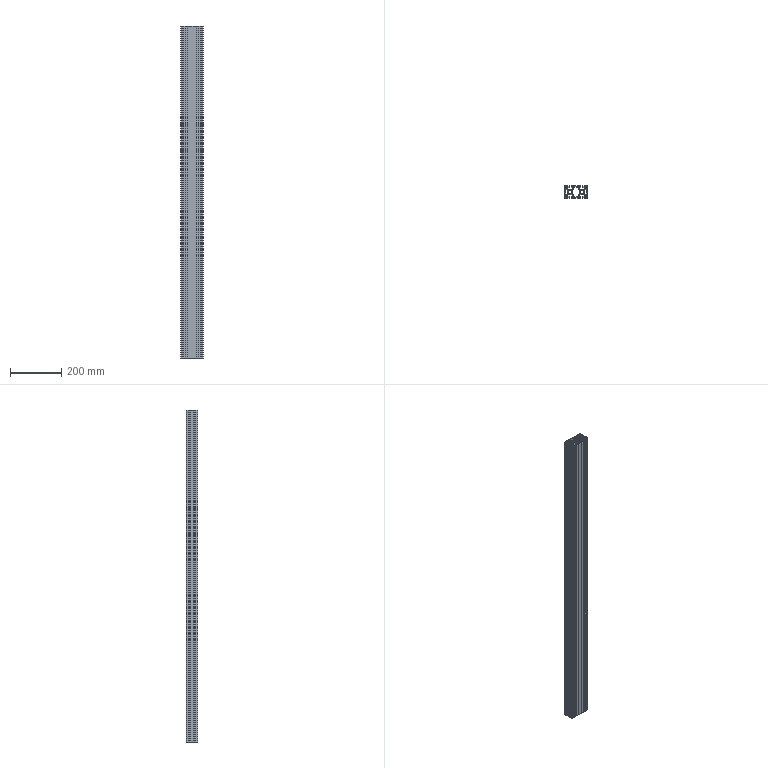Part | STEP file | 4590-1300 | 1 solid | 366 faces | box 90 x 45 x 1300 mm | volume 1524515 mm3 | plane 254 | cylinder 112 | commonest cylinder face diameters 2 x64 8 x20 12 x16 4 x12